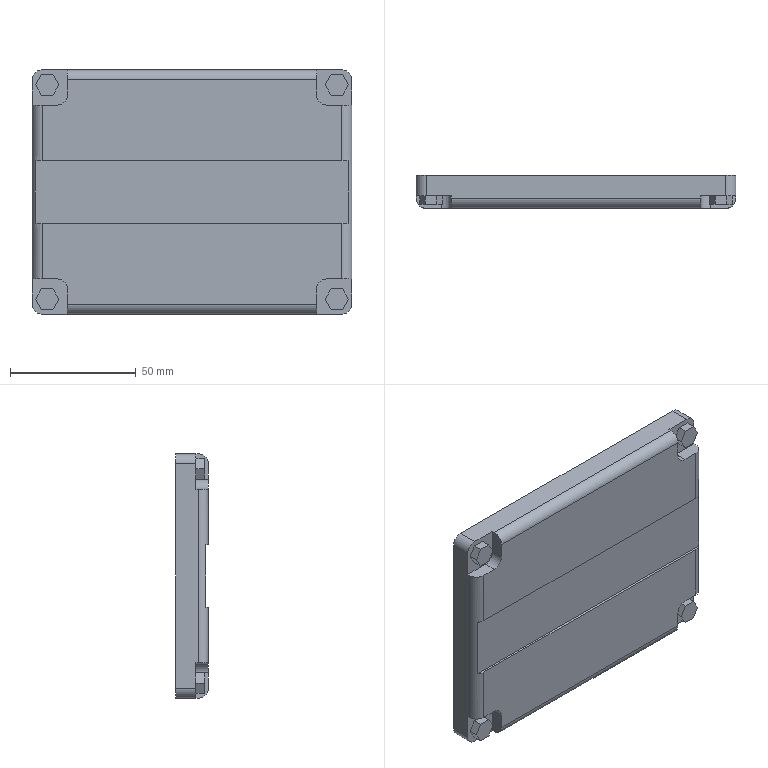Part | SolidWorks | features BaseBody 1 | 1 solid | 62 faces | box 127 x 13 x 97 mm | volume 152742 mm3 | plane 50 | cylinder 12 | commonest cylinder face diameters 8 x12